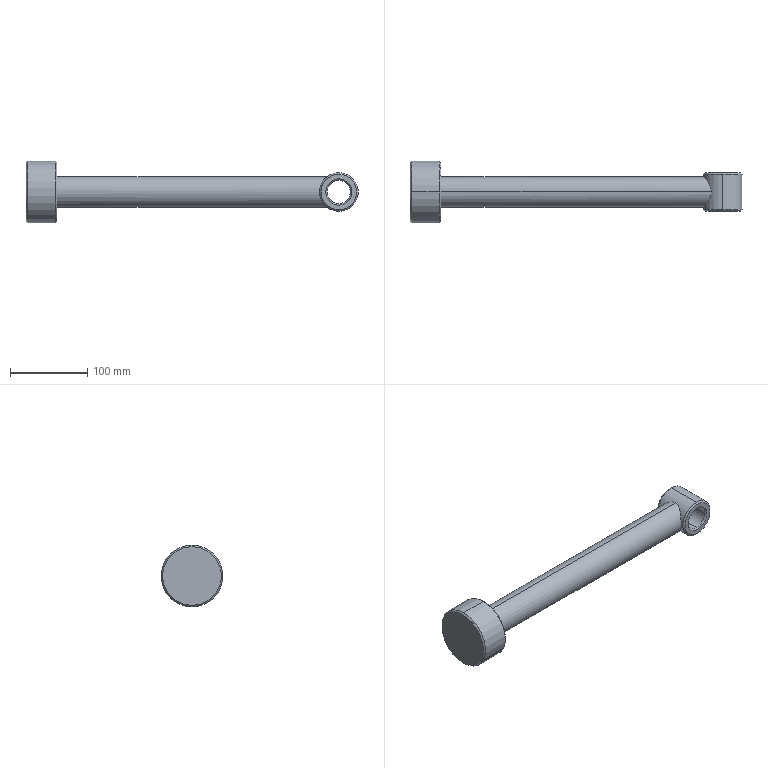Part | STEP file | Piston rod | 1 solid | 24 faces | box 430 x 80 x 80 mm | volume 691930 mm3 | cone 12 | cylinder 8 | plane 4 | commonest cylinder face diameters 30 x2 40 x2 50 x2 80 x2
STEP:
#1=CARTESIAN_POINT('',(405.,-23.,15.));
#2=VERTEX_POINT('',#1);
#3=CARTESIAN_POINT('',(405.,-23.,-15.));
#4=VERTEX_POINT('',#3);
#5=CARTESIAN_POINT('',(405.,-23.,0.));
#6=DIRECTION('',(0.,-1.,0.));
#7=DIRECTION('',(0.,0.,1.));
#8=AXIS2_PLACEMENT_3D('',#5,#6,#7);
#9=CIRCLE('',#8,15.);
#10=EDGE_CURVE('',#2,#4,#9,.T.);
#11=ORIENTED_EDGE('',*,*,#10,.F.);
#12=CARTESIAN_POINT('',(405.,-25.,17.));
#13=VERTEX_POINT('',#12);
#14=CARTESIAN_POINT('',(405.,-25.,17.));
#15=DIRECTION('',(0.,-0.7071,0.7071));
#16=VECTOR('',#15,1000.);
#17=LINE('',#14,#16);
#18=EDGE_CURVE('',#2,#13,#17,.T.);
#19=ORIENTED_EDGE('',*,*,#18,.T.);
#20=CARTESIAN_POINT('',(405.,-25.,-17.));
#21=VERTEX_POINT('',#20);
#22=CARTESIAN_POINT('',(405.,-25.,0.));
#23=DIRECTION('',(0.,1.,0.));
#24=DIRECTION('',(0.,0.,1.));
#25=AXIS2_PLACEMENT_3D('',#22,#23,#24);
#26=CIRCLE('',#25,17.);
#27=EDGE_CURVE('',#21,#13,#26,.T.);
#28=ORIENTED_EDGE('',*,*,#27,.F.);
#29=CARTESIAN_POINT('',(405.,-25.,-17.));
#30=DIRECTION('',(0.,-0.7071,-0.7071));
#31=VECTOR('',#30,1000.);
#32=LINE('',#29,#31);
#33=EDGE_CURVE('',#4,#21,#32,.T.);
#34=ORIENTED_EDGE('',*,*,#33,.F.);
#35=EDGE_LOOP('',(#11,#19,#28,#34));
#36=FACE_OUTER_BOUND('',#35,.T.);
#37=CARTESIAN_POINT('',(405.,-25.,0.));
#38=DIRECTION('',(0.,-1.,0.));
#39=DIRECTION('',(0.,0.,-1.));
#40=AXIS2_PLACEMENT_3D('',#37,#38,#39);
#41=CONICAL_SURFACE('',#40,17.,0.7854);
#42=ADVANCED_FACE('',(#36),#41,.F.);
#43=CARTESIAN_POINT('',(405.,-25.,-23.));
#44=VERTEX_POINT('',#43);
#45=CARTESIAN_POINT('',(405.,-25.,23.));
#46=VERTEX_POINT('',#45);
#47=CARTESIAN_POINT('',(405.,-25.,0.));
#48=DIRECTION('',(0.,-1.,0.));
#49=DIRECTION('',(0.,0.,1.));
#50=AXIS2_PLACEMENT_3D('',#47,#48,#49);
#51=CIRCLE('',#50,23.);
#52=EDGE_CURVE('',#44,#46,#51,.T.);
#53=ORIENTED_EDGE('',*,*,#52,.F.);
#54=CARTESIAN_POINT('',(405.,-23.,-25.));
#55=VERTEX_POINT('',#54);
#56=CARTESIAN_POINT('',(405.,-23.,-25.));
#57=DIRECTION('',(0.,0.7071,-0.7071));
#58=VECTOR('',#57,1000.);
#59=LINE('',#56,#58);
#60=EDGE_CURVE('',#44,#55,#59,.T.);
#61=ORIENTED_EDGE('',*,*,#60,.T.);
#62=CARTESIAN_POINT('',(405.,-23.,25.));
#63=VERTEX_POINT('',#62);
#64=CARTESIAN_POINT('',(405.,-23.,0.));
#65=DIRECTION('',(0.,1.,0.));
#66=DIRECTION('',(0.,0.,1.));
#67=AXIS2_PLACEMENT_3D('',#64,#65,#66);
#68=CIRCLE('',#67,25.);
#69=EDGE_CURVE('',#63,#55,#68,.T.);
#70=ORIENTED_EDGE('',*,*,#69,.F.);
#71=CARTESIAN_POINT('',(405.,-23.,25.));
#72=DIRECTION('',(0.,0.7071,0.7071));
#73=VECTOR('',#72,1000.);
#74=LINE('',#71,#73);
#75=EDGE_CURVE('',#46,#63,#74,.T.);
#76=ORIENTED_EDGE('',*,*,#75,.F.);
#77=EDGE_LOOP('',(#53,#61,#70,#76));
#78=FACE_OUTER_BOUND('',#77,.T.);
#79=CARTESIAN_POINT('',(405.,-23.,0.));
#80=DIRECTION('',(0.,1.,0.));
#81=DIRECTION('',(0.,0.,1.));
#82=AXIS2_PLACEMENT_3D('',#79,#80,#81);
#83=CONICAL_SURFACE('',#82,25.,0.7854);
#84=ADVANCED_FACE('',(#78),#83,.T.);
#85=CARTESIAN_POINT('',(405.,25.,23.));
#86=VERTEX_POINT('',#85);
#87=CARTESIAN_POINT('',(405.,25.,-23.));
#88=VERTEX_POINT('',#87);
#89=CARTESIAN_POINT('',(405.,25.,0.));
#90=DIRECTION('',(0.,1.,0.));
#91=DIRECTION('',(0.,0.,1.));
#92=AXIS2_PLACEMENT_3D('',#89,#90,#91);
#93=CIRCLE('',#92,23.);
#94=EDGE_CURVE('',#86,#88,#93,.T.);
#95=ORIENTED_EDGE('',*,*,#94,.F.);
#96=CARTESIAN_POINT('',(405.,23.,25.));
#97=VERTEX_POINT('',#96);
#98=CARTESIAN_POINT('',(405.,25.,23.));
#99=DIRECTION('',(0.,-0.7071,0.7071));
#100=VECTOR('',#99,1000.);
#101=LINE('',#98,#100);
#102=EDGE_CURVE('',#86,#97,#101,.T.);
#103=ORIENTED_EDGE('',*,*,#102,.T.);
#104=CARTESIAN_POINT('',(405.,23.,-25.));
#105=VERTEX_POINT('',#104);
#106=CARTESIAN_POINT('',(405.,23.,0.));
#107=DIRECTION('',(0.,-1.,0.));
#108=DIRECTION('',(0.,0.,1.));
#109=AXIS2_PLACEMENT_3D('',#106,#107,#108);
#110=CIRCLE('',#109,25.);
#111=EDGE_CURVE('',#105,#97,#110,.T.);
#112=ORIENTED_EDGE('',*,*,#111,.F.);
#113=CARTESIAN_POINT('',(405.,25.,-23.));
#114=DIRECTION('',(0.,-0.7071,-0.7071));
#115=VECTOR('',#114,1000.);
#116=LINE('',#113,#115);
#117=EDGE_CURVE('',#88,#105,#116,.T.);
#118=ORIENTED_EDGE('',*,*,#117,.F.);
#119=EDGE_LOOP('',(#95,#103,#112,#118));
#120=FACE_OUTER_BOUND('',#119,.T.);
#121=CARTESIAN_POINT('',(405.,25.,0.));
#122=DIRECTION('',(0.,-1.,0.));
#123=DIRECTION('',(0.,0.,-1.));
#124=AXIS2_PLACEMENT_3D('',#121,#122,#123);
#125=CONICAL_SURFACE('',#124,23.,0.7854);
#126=ADVANCED_FACE('',(#120),#125,.T.);
#127=CARTESIAN_POINT('',(405.,23.,-15.));
#128=VERTEX_POINT('',#127);
#129=CARTESIAN_POINT('',(405.,23.,15.));
#130=VERTEX_POINT('',#129);
#131=CARTESIAN_POINT('',(405.,23.,0.));
#132=DIRECTION('',(0.,1.,0.));
#133=DIRECTION('',(0.,0.,1.));
#134=AXIS2_PLACEMENT_3D('',#131,#132,#133);
#135=CIRCLE('',#134,15.);
#136=EDGE_CURVE('',#128,#130,#135,.T.);
#137=ORIENTED_EDGE('',*,*,#136,.F.);
#138=CARTESIAN_POINT('',(405.,25.,-17.));
#139=VERTEX_POINT('',#138);
#140=CARTESIAN_POINT('',(405.,23.,-15.));
#141=DIRECTION('',(0.,0.7071,-0.7071));
#142=VECTOR('',#141,1000.);
#143=LINE('',#140,#142);
#144=EDGE_CURVE('',#128,#139,#143,.T.);
#145=ORIENTED_EDGE('',*,*,#144,.T.);
#146=CARTESIAN_POINT('',(405.,25.,17.));
#147=VERTEX_POINT('',#146);
#148=CARTESIAN_POINT('',(405.,25.,0.));
#149=DIRECTION('',(0.,-1.,0.));
#150=DIRECTION('',(0.,0.,1.));
#151=AXIS2_PLACEMENT_3D('',#148,#149,#150);
#152=CIRCLE('',#151,17.);
#153=EDGE_CURVE('',#147,#139,#152,.T.);
#154=ORIENTED_EDGE('',*,*,#153,.F.);
#155=CARTESIAN_POINT('',(405.,23.,15.));
#156=DIRECTION('',(0.,0.7071,0.7071));
#157=VECTOR('',#156,1000.);
#158=LINE('',#155,#157);
#159=EDGE_CURVE('',#130,#147,#158,.T.);
#160=ORIENTED_EDGE('',*,*,#159,.F.);
#161=EDGE_LOOP('',(#137,#145,#154,#160));
#162=FACE_OUTER_BOUND('',#161,.T.);
#163=CARTESIAN_POINT('',(405.,23.,0.));
#164=DIRECTION('',(0.,1.,0.));
#165=DIRECTION('',(0.,0.,1.));
#166=AXIS2_PLACEMENT_3D('',#163,#164,#165);
#167=CONICAL_SURFACE('',#166,15.,0.7854);
#168=ADVANCED_FACE('',(#162),#167,.F.);
#169=CARTESIAN_POINT('',(40.,0.,-38.));
#170=VERTEX_POINT('',#169);
#171=CARTESIAN_POINT('',(40.,0.,38.));
#172=VERTEX_POINT('',#171);
#173=CARTESIAN_POINT('',(40.,0.,0.));
#174=DIRECTION('',(1.,0.,0.));
#175=DIRECTION('',(0.,0.,1.));
#176=AXIS2_PLACEMENT_3D('',#173,#174,#175);
#177=CIRCLE('',#176,38.);
#178=EDGE_CURVE('',#170,#172,#177,.T.);
#179=ORIENTED_EDGE('',*,*,#178,.F.);
#180=CARTESIAN_POINT('',(38.,0.,-40.));
#181=VERTEX_POINT('',#180);
#182=CARTESIAN_POINT('',(38.,0.,-40.));
#183=DIRECTION('',(-0.7071,0.,-0.7071));
#184=VECTOR('',#183,1000.);
#185=LINE('',#182,#184);
#186=EDGE_CURVE('',#170,#181,#185,.T.);
#187=ORIENTED_EDGE('',*,*,#186,.T.);
#188=CARTESIAN_POINT('',(38.,0.,40.));
#189=VERTEX_POINT('',#188);
#190=CARTESIAN_POINT('',(38.,0.,0.));
#191=DIRECTION('',(-1.,0.,0.));
#192=DIRECTION('',(0.,0.,1.));
#193=AXIS2_PLACEMENT_3D('',#190,#191,#192);
#194=CIRCLE('',#193,40.);
#195=EDGE_CURVE('',#189,#181,#194,.T.);
#196=ORIENTED_EDGE('',*,*,#195,.F.);
#197=CARTESIAN_POINT('',(38.,0.,40.));
#198=DIRECTION('',(-0.7071,0.,0.7071));
#199=VECTOR('',#198,1000.);
#200=LINE('',#197,#199);
#201=EDGE_CURVE('',#172,#189,#200,.T.);
#202=ORIENTED_EDGE('',*,*,#201,.F.);
#203=EDGE_LOOP('',(#179,#187,#196,#202));
#204=FACE_OUTER_BOUND('',#203,.T.);
#205=CARTESIAN_POINT('',(38.,0.,0.));
#206=DIRECTION('',(-1.,0.,0.));
#207=DIRECTION('',(0.,0.,1.));
#208=AXIS2_PLACEMENT_3D('',#205,#206,#207);
#209=CONICAL_SURFACE('',#208,40.,0.7854);
#210=ADVANCED_FACE('',(#204),#209,.T.);
#211=CARTESIAN_POINT('',(0.,0.,38.));
#212=VERTEX_POINT('',#211);
#213=CARTESIAN_POINT('',(0.,0.,-38.));
#214=VERTEX_POINT('',#213);
#215=CARTESIAN_POINT('',(0.,0.,0.));
#216=DIRECTION('',(-1.,0.,0.));
#217=DIRECTION('',(0.,0.,-1.));
#218=AXIS2_PLACEMENT_3D('',#215,#216,#217);
#219=CIRCLE('',#218,38.);
#220=EDGE_CURVE('',#212,#214,#219,.T.);
#221=ORIENTED_EDGE('',*,*,#220,.F.);
#222=CARTESIAN_POINT('',(2.,0.,40.));
#223=VERTEX_POINT('',#222);
#224=CARTESIAN_POINT('',(0.,0.,38.));
#225=DIRECTION('',(0.7071,0.,0.7071));
#226=VECTOR('',#225,1000.);
#227=LINE('',#224,#226);
#228=EDGE_CURVE('',#212,#223,#227,.T.);
#229=ORIENTED_EDGE('',*,*,#228,.T.);
#230=CARTESIAN_POINT('',(2.,0.,-40.));
#231=VERTEX_POINT('',#230);
#232=CARTESIAN_POINT('',(2.,0.,0.));
#233=DIRECTION('',(1.,0.,0.));
#234=DIRECTION('',(0.,0.,-1.));
#235=AXIS2_PLACEMENT_3D('',#232,#233,#234);
#236=CIRCLE('',#235,40.);
#237=EDGE_CURVE('',#231,#223,#236,.T.);
#238=ORIENTED_EDGE('',*,*,#237,.F.);
#239=CARTESIAN_POINT('',(0.,0.,-38.));
#240=DIRECTION('',(0.7071,0.,-0.7071));
#241=VECTOR('',#240,1000.);
#242=LINE('',#239,#241);
#243=EDGE_CURVE('',#214,#231,#242,.T.);
#244=ORIENTED_EDGE('',*,*,#243,.F.);
#245=EDGE_LOOP('',(#221,#229,#238,#244));
#246=FACE_OUTER_BOUND('',#245,.T.);
#247=CARTESIAN_POINT('',(0.,0.,0.));
#248=DIRECTION('',(1.,0.,0.));
#249=DIRECTION('',(0.,0.,-1.));
#250=AXIS2_PLACEMENT_3D('',#247,#248,#249);
#251=CONICAL_SURFACE('',#250,38.,0.7854);
#252=ADVANCED_FACE('',(#246),#251,.T.);
#253=ORIENTED_EDGE('',*,*,#10,.T.);
#254=CARTESIAN_POINT('',(405.,-25.,-15.));
#255=DIRECTION('',(0.,1.,0.));
#256=VECTOR('',#255,1000.);
#257=LINE('',#254,#256);
#258=EDGE_CURVE('',#4,#128,#257,.T.);
#259=ORIENTED_EDGE('',*,*,#258,.T.);
#260=ORIENTED_EDGE('',*,*,#136,.T.);
#261=CARTESIAN_POINT('',(405.,-25.,15.));
#262=DIRECTION('',(0.,1.,0.));
#263=VECTOR('',#262,1000.);
#264=LINE('',#261,#263);
#265=EDGE_CURVE('',#2,#130,#264,.T.);
#266=ORIENTED_EDGE('',*,*,#265,.F.);
#267=EDGE_LOOP('',(#253,#259,#260,#266));
#268=FACE_OUTER_BOUND('',#267,.T.);
#269=CARTESIAN_POINT('',(405.,-25.,0.));
#270=DIRECTION('',(0.,1.,0.));
#271=DIRECTION('',(0.,0.,1.));
#272=AXIS2_PLACEMENT_3D('',#269,#270,#271);
#273=CYLINDRICAL_SURFACE('',#272,15.);
#274=ADVANCED_FACE('',(#268),#273,.F.);
#275=ORIENTED_EDGE('',*,*,#69,.T.);
#276=CARTESIAN_POINT('',(405.,-25.,-25.));
#277=DIRECTION('',(0.,1.,0.));
#278=VECTOR('',#277,1000.);
#279=LINE('',#276,#278);
#280=EDGE_CURVE('',#55,#105,#279,.T.);
#281=ORIENTED_EDGE('',*,*,#280,.T.);
#282=ORIENTED_EDGE('',*,*,#111,.T.);
#283=CARTESIAN_POINT('',(405.,-25.,25.));
#284=DIRECTION('',(0.,1.,0.));
#285=VECTOR('',#284,1000.);
#286=LINE('',#283,#285);
#287=EDGE_CURVE('',#63,#97,#286,.T.);
#288=ORIENTED_EDGE('',*,*,#287,.F.);
#289=EDGE_LOOP('',(#275,#281,#282,#288));
#290=FACE_OUTER_BOUND('',#289,.T.);
#291=CARTESIAN_POINT('',(405.,-25.,0.));
#292=DIRECTION('',(0.,1.,0.));
#293=DIRECTION('',(0.,0.,1.));
#294=AXIS2_PLACEMENT_3D('',#291,#292,#293);
#295=CYLINDRICAL_SURFACE('',#294,25.);
#296=ADVANCED_FACE('',(#290),#295,.T.);
#297=CARTESIAN_POINT('',(390.,0.,20.));
#298=VERTEX_POINT('',#297);
#299=CARTESIAN_POINT('',(390.,0.,-20.));
#300=VERTEX_POINT('',#299);
#301=CARTESIAN_POINT('',(390.,0.,20.));
#302=CARTESIAN_POINT('',(390.,1.405,20.));
#303=CARTESIAN_POINT('',(389.801,2.765,19.854));
#304=CARTESIAN_POINT('',(389.366,4.419,19.509));
#305=CARTESIAN_POINT('',(389.27,4.748,19.431));
#306=CARTESIAN_POINT('',(389.064,5.391,19.263));
#307=CARTESIAN_POINT('',(388.954,5.707,19.171));
#308=CARTESIAN_POINT('',(388.606,6.639,18.877));
#309=CARTESIAN_POINT('',(388.352,7.241,18.654));
#310=CARTESIAN_POINT('',(387.81,8.412,18.156));
#311=CARTESIAN_POINT('',(387.524,8.98,17.882));
#312=CARTESIAN_POINT('',(386.929,10.089,17.281));
#313=CARTESIAN_POINT('',(386.624,10.624,16.957));
#314=CARTESIAN_POINT('',(385.704,12.167,15.922));
#315=CARTESIAN_POINT('',(385.083,13.119,15.147));
#316=CARTESIAN_POINT('',(384.176,14.448,13.844));
#317=CARTESIAN_POINT('',(383.878,14.873,13.386));
#318=CARTESIAN_POINT('',(383.295,15.69,12.418));
#319=CARTESIAN_POINT('',(383.013,16.078,11.913));
#320=CARTESIAN_POINT('',(382.208,17.167,10.341));
#321=CARTESIAN_POINT('',(381.725,17.8,9.215));
#322=CARTESIAN_POINT('',(381.21,18.465,7.692));
#323=CARTESIAN_POINT('',(381.112,18.592,7.38));
#324=CARTESIAN_POINT('',(380.927,18.829,6.751));
#325=CARTESIAN_POINT('',(380.84,18.94,6.433));
#326=CARTESIAN_POINT('',(380.597,19.249,5.471));
#327=CARTESIAN_POINT('',(380.459,19.423,4.817));
#328=CARTESIAN_POINT('',(380.235,19.706,3.483));
#329=CARTESIAN_POINT('',(380.148,19.815,2.803));
#330=CARTESIAN_POINT('',(380.03,19.962,1.415));
#331=CARTESIAN_POINT('',(380.001,19.999,0.7219));
#332=CARTESIAN_POINT('',(379.999,20.001,-0.6588));
#333=CARTESIAN_POINT('',(380.027,19.967,-1.347));
#334=CARTESIAN_POINT('',(380.111,19.861,-2.376));
#335=CARTESIAN_POINT('',(380.146,19.817,-2.719));
#336=CARTESIAN_POINT('',(380.23,19.711,-3.403));
#337=CARTESIAN_POINT('',(380.28,19.649,-3.745));
#338=CARTESIAN_POINT('',(380.558,19.298,-5.428));
#339=CARTESIAN_POINT('',(380.883,18.888,-6.71));
#340=CARTESIAN_POINT('',(381.394,18.227,-8.239));
#341=CARTESIAN_POINT('',(381.502,18.087,-8.541));
#342=CARTESIAN_POINT('',(381.726,17.796,-9.134));
#343=CARTESIAN_POINT('',(381.842,17.644,-9.424));
#344=CARTESIAN_POINT('',(382.202,17.17,-10.278));
#345=CARTESIAN_POINT('',(382.457,16.83,-10.824));
#346=CARTESIAN_POINT('',(382.993,16.105,-11.877));
#347=CARTESIAN_POINT('',(383.274,15.719,-12.382));
#348=CARTESIAN_POINT('',(383.858,14.903,-13.354));
#349=CARTESIAN_POINT('',(384.157,14.476,-13.815));
#350=CARTESIAN_POINT('',(385.066,13.144,-15.125));
#351=CARTESIAN_POINT('',(385.69,12.188,-15.906));
#352=CARTESIAN_POINT('',(386.616,10.636,-16.949));
#353=CARTESIAN_POINT('',(386.924,10.098,-17.275));
#354=CARTESIAN_POINT('',(387.516,8.995,-17.874));
#355=CARTESIAN_POINT('',(387.802,8.428,-18.149));
#356=CARTESIAN_POINT('',(388.344,7.258,-18.648));
#357=CARTESIAN_POINT('',(388.6,6.655,-18.872));
#358=CARTESIAN_POINT('',(389.066,5.406,-19.267));
#359=CARTESIAN_POINT('',(389.277,4.756,-19.438));
#360=CARTESIAN_POINT('',(389.624,3.439,-19.714));
#361=CARTESIAN_POINT('',(389.762,2.768,-19.819));
#362=CARTESIAN_POINT('',(389.903,1.742,-19.927));
#363=CARTESIAN_POINT('',(389.939,1.397,-19.954));
#364=CARTESIAN_POINT('',(389.988,0.698,-19.991));
#365=CARTESIAN_POINT('',(390.,0.3476,-20.));
#366=CARTESIAN_POINT('',(390.,0.,-20.));
#367=B_SPLINE_CURVE_WITH_KNOTS('',3,(#301,#302,#303,#304,#305,#306,#307,#308,#309,#310,#311,#312,#313,#314,#315,#316,#317,#318,#319,#320,#321,#322,#323,#324,#325,#326,#327,#328,#329,#330,#331,#332,#333,#334,#335,#336,#337,#338,#339,#340,#341,#342,#343,#344,#345,#346,#347,#348,#349,#350,#351,#352,#353,#354,#355,#356,#357,#358,#359,#360,#361,#362,#363,#364,#365,#366),.UNSPECIFIED.,.F.,.F.,(4,2,2,2,2,2,2,2,2,2,2,2,2,2,2,2,2,2,2,2,2,2,2,2,2,2,2,2,2,2,2,2,4),(0.,0.004146,0.005182,0.006219,0.008292,0.01036,0.01244,0.01658,0.01866,0.02073,0.02487,0.02591,0.02695,0.02902,0.03109,0.03317,0.03524,0.03628,0.03731,0.04146,0.04249,0.04353,0.0456,0.04768,0.04975,0.0539,0.05597,0.05804,0.06011,0.06219,0.06426,0.0653,0.06633),.UNSPECIFIED.);
#368=EDGE_CURVE('',#298,#300,#367,.T.);
#369=ORIENTED_EDGE('',*,*,#368,.T.);
#370=CARTESIAN_POINT('',(40.,0.,-20.));
#371=VERTEX_POINT('',#370);
#372=CARTESIAN_POINT('',(0.,0.,-20.));
#373=DIRECTION('',(-1.,0.,0.));
#374=VECTOR('',#373,1000.);
#375=LINE('',#372,#374);
#376=EDGE_CURVE('',#300,#371,#375,.T.);
#377=ORIENTED_EDGE('',*,*,#376,.T.);
#378=CARTESIAN_POINT('',(40.,0.,20.));
#379=VERTEX_POINT('',#378);
#380=CARTESIAN_POINT('',(40.,0.,0.));
#381=DIRECTION('',(-1.,0.,0.));
#382=DIRECTION('',(0.,0.,1.));
#383=AXIS2_PLACEMENT_3D('',#380,#381,#382);
#384=CIRCLE('',#383,20.);
#385=EDGE_CURVE('',#379,#371,#384,.T.);
#386=ORIENTED_EDGE('',*,*,#385,.F.);
#387=CARTESIAN_POINT('',(0.,0.,20.));
#388=DIRECTION('',(-1.,0.,0.));
#389=VECTOR('',#388,1000.);
#390=LINE('',#387,#389);
#391=EDGE_CURVE('',#298,#379,#390,.T.);
#392=ORIENTED_EDGE('',*,*,#391,.F.);
#393=EDGE_LOOP('',(#369,#377,#386,#392));
#394=FACE_OUTER_BOUND('',#393,.T.);
#395=CARTESIAN_POINT('',(0.,0.,0.));
#396=DIRECTION('',(-1.,0.,0.));
#397=DIRECTION('',(0.,0.,1.));
#398=AXIS2_PLACEMENT_3D('',#395,#396,#397);
#399=CYLINDRICAL_SURFACE('',#398,20.);
#400=ADVANCED_FACE('',(#394),#399,.T.);
#401=ORIENTED_EDGE('',*,*,#195,.T.);
#402=CARTESIAN_POINT('',(0.,0.,-40.));
#403=DIRECTION('',(-1.,0.,0.));
#404=VECTOR('',#403,1000.);
#405=LINE('',#402,#404);
#406=EDGE_CURVE('',#181,#231,#405,.T.);
#407=ORIENTED_EDGE('',*,*,#406,.T.);
#408=ORIENTED_EDGE('',*,*,#237,.T.);
#409=CARTESIAN_POINT('',(0.,0.,40.));
#410=DIRECTION('',(-1.,0.,0.));
#411=VECTOR('',#410,1000.);
#412=LINE('',#409,#411);
#413=EDGE_CURVE('',#189,#223,#412,.T.);
#414=ORIENTED_EDGE('',*,*,#413,.F.);
#415=EDGE_LOOP('',(#401,#407,#408,#414));
#416=FACE_OUTER_BOUND('',#415,.T.);
#417=CARTESIAN_POINT('',(0.,0.,0.));
#418=DIRECTION('',(-1.,0.,0.));
#419=DIRECTION('',(0.,0.,1.));
#420=AXIS2_PLACEMENT_3D('',#417,#418,#419);
#421=CYLINDRICAL_SURFACE('',#420,40.);
#422=ADVANCED_FACE('',(#416),#421,.T.);
#423=CARTESIAN_POINT('',(0.,0.,0.));
#424=DIRECTION('',(-1.,0.,0.));
#425=DIRECTION('',(0.,0.,-1.));
#426=AXIS2_PLACEMENT_3D('',#423,#424,#425);
#427=CIRCLE('',#426,38.);
#428=EDGE_CURVE('',#214,#212,#427,.T.);
#429=ORIENTED_EDGE('',*,*,#428,.T.);
#430=ORIENTED_EDGE('',*,*,#220,.T.);
#431=EDGE_LOOP('',(#429,#430));
#432=FACE_OUTER_BOUND('',#431,.T.);
#433=CARTESIAN_POINT('',(0.,0.,0.));
#434=DIRECTION('',(1.,0.,0.));
#435=DIRECTION('',(0.,0.,-1.));
#436=AXIS2_PLACEMENT_3D('',#433,#434,#435);
#437=PLANE('',#436);
#438=ADVANCED_FACE('',(#432),#437,.F.);
#439=ORIENTED_EDGE('',*,*,#406,.F.);
#440=CARTESIAN_POINT('',(38.,0.,0.));
#441=DIRECTION('',(-1.,0.,0.));
#442=DIRECTION('',(0.,0.,1.));
#443=AXIS2_PLACEMENT_3D('',#440,#441,#442);
#444=CIRCLE('',#443,40.);
#445=EDGE_CURVE('',#181,#189,#444,.T.);
#446=ORIENTED_EDGE('',*,*,#445,.T.);
#447=ORIENTED_EDGE('',*,*,#413,.T.);
#448=CARTESIAN_POINT('',(2.,0.,0.));
#449=DIRECTION('',(1.,0.,0.));
#450=DIRECTION('',(0.,0.,-1.));
#451=AXIS2_PLACEMENT_3D('',#448,#449,#450);
#452=CIRCLE('',#451,40.);
#453=EDGE_CURVE('',#223,#231,#452,.T.);
#454=ORIENTED_EDGE('',*,*,#453,.T.);
#455=EDGE_LOOP('',(#439,#446,#447,#454));
#456=FACE_OUTER_BOUND('',#455,.T.);
#457=CARTESIAN_POINT('',(0.,0.,0.));
#458=DIRECTION('',(-1.,0.,0.));
#459=DIRECTION('',(0.,0.,1.));
#460=AXIS2_PLACEMENT_3D('',#457,#458,#459);
#461=CYLINDRICAL_SURFACE('',#460,40.);
#462=ADVANCED_FACE('',(#456),#461,.T.);
#463=CARTESIAN_POINT('',(40.,0.,0.));
#464=DIRECTION('',(1.,0.,0.));
#465=DIRECTION('',(0.,0.,1.));
#466=AXIS2_PLACEMENT_3D('',#463,#464,#465);
#467=CIRCLE('',#466,38.);
#468=EDGE_CURVE('',#172,#170,#467,.T.);
#469=ORIENTED_EDGE('',*,*,#468,.T.);
#470=ORIENTED_EDGE('',*,*,#178,.T.);
#471=EDGE_LOOP('',(#469,#470));
#472=FACE_OUTER_BOUND('',#471,.T.);
#473=ORIENTED_EDGE('',*,*,#385,.T.);
#474=CARTESIAN_POINT('',(40.,0.,0.));
#475=DIRECTION('',(-1.,0.,0.));
#476=DIRECTION('',(0.,0.,1.));
#477=AXIS2_PLACEMENT_3D('',#474,#475,#476);
#478=CIRCLE('',#477,20.);
#479=EDGE_CURVE('',#371,#379,#478,.T.);
#480=ORIENTED_EDGE('',*,*,#479,.T.);
#481=EDGE_LOOP('',(#473,#480));
#482=FACE_BOUND('',#481,.T.);
#483=CARTESIAN_POINT('',(40.,40.,0.));
#484=DIRECTION('',(-1.,0.,0.));
#485=DIRECTION('',(0.,0.,1.));
#486=AXIS2_PLACEMENT_3D('',#483,#484,#485);
#487=PLANE('',#486);
#488=ADVANCED_FACE('',(#472,#482),#487,.F.);
#489=ORIENTED_EDGE('',*,*,#376,.F.);
#490=CARTESIAN_POINT('',(390.,0.,-20.));
#491=CARTESIAN_POINT('',(390.,-0.6946,-20.));
#492=CARTESIAN_POINT('',(389.952,-1.383,-19.964));
#493=CARTESIAN_POINT('',(389.812,-2.406,-19.858));
#494=CARTESIAN_POINT('',(389.754,-2.745,-19.814));
#495=CARTESIAN_POINT('',(389.618,-3.421,-19.708));
#496=CARTESIAN_POINT('',(389.54,-3.758,-19.647));
#497=CARTESIAN_POINT('',(389.106,-5.409,-19.302));
#498=CARTESIAN_POINT('',(388.628,-6.644,-18.908));
#499=CARTESIAN_POINT('',(387.812,-8.409,-18.158));
#500=CARTESIAN_POINT('',(387.522,-8.983,-17.88));
#501=CARTESIAN_POINT('',(386.931,-10.085,-17.283));
#502=CARTESIAN_POINT('',(386.628,-10.615,-16.962));
#503=CARTESIAN_POINT('',(385.712,-12.154,-15.932));
#504=CARTESIAN_POINT('',(385.09,-13.109,-15.156));
#505=CARTESIAN_POINT('',(384.177,-14.447,-13.845));
#506=CARTESIAN_POINT('',(383.876,-14.877,-13.382));
#507=CARTESIAN_POINT('',(383.298,-15.687,-12.423));
#508=CARTESIAN_POINT('',(383.019,-16.069,-11.924));
#509=CARTESIAN_POINT('',(382.22,-17.151,-10.366));
#510=CARTESIAN_POINT('',(381.737,-17.784,-9.247));
#511=CARTESIAN_POINT('',(381.221,-18.451,-7.725));
#512=CARTESIAN_POINT('',(381.122,-18.578,-7.414));
#513=CARTESIAN_POINT('',(380.936,-18.817,-6.785));
#514=CARTESIAN_POINT('',(380.849,-18.928,-6.468));
#515=CARTESIAN_POINT('',(380.605,-19.239,-5.505));
#516=CARTESIAN_POINT('',(380.466,-19.415,-4.851));
#517=CARTESIAN_POINT('',(380.239,-19.7,-3.517));
#518=CARTESIAN_POINT('',(380.152,-19.81,-2.835));
#519=CARTESIAN_POINT('',(380.032,-19.96,-1.447));
#520=CARTESIAN_POINT('',(380.002,-19.998,-0.7543));
#521=CARTESIAN_POINT('',(379.998,-20.002,0.6273));
#522=CARTESIAN_POINT('',(380.025,-19.969,1.316));
#523=CARTESIAN_POINT('',(380.108,-19.865,2.347));
#524=CARTESIAN_POINT('',(380.143,-19.821,2.69));
#525=CARTESIAN_POINT('',(380.227,-19.716,3.376));
#526=CARTESIAN_POINT('',(380.276,-19.654,3.718));
#527=CARTESIAN_POINT('',(380.553,-19.306,5.403));
#528=CARTESIAN_POINT('',(380.876,-18.897,6.686));
#529=CARTESIAN_POINT('',(381.387,-18.237,8.218));
#530=CARTESIAN_POINT('',(381.495,-18.097,8.521));
#531=CARTESIAN_POINT('',(381.718,-17.806,9.114));
#532=CARTESIAN_POINT('',(381.834,-17.654,9.405));
#533=CARTESIAN_POINT('',(382.194,-17.18,10.26));
#534=CARTESIAN_POINT('',(382.449,-16.841,10.807));
#535=CARTESIAN_POINT('',(382.985,-16.116,11.862));
#536=CARTESIAN_POINT('',(383.266,-15.73,12.368));
#537=CARTESIAN_POINT('',(383.85,-14.913,13.342));
#538=CARTESIAN_POINT('',(384.149,-14.487,13.803));
#539=CARTESIAN_POINT('',(385.059,-13.156,15.116));
#540=CARTESIAN_POINT('',(385.684,-12.199,15.898));
#541=CARTESIAN_POINT('',(386.611,-10.646,16.943));
#542=CARTESIAN_POINT('',(386.918,-10.107,17.269));
#543=CARTESIAN_POINT('',(387.511,-9.004,17.869));
#544=CARTESIAN_POINT('',(387.798,-8.437,18.144));
#545=CARTESIAN_POINT('',(388.341,-7.267,18.644));
#546=CARTESIAN_POINT('',(388.597,-6.664,18.869));
#547=CARTESIAN_POINT('',(389.064,-5.413,19.265));
#548=CARTESIAN_POINT('',(389.275,-4.763,19.436));
#549=CARTESIAN_POINT('',(389.622,-3.446,19.712));
#550=CARTESIAN_POINT('',(389.761,-2.775,19.818));
#551=CARTESIAN_POINT('',(389.902,-1.748,19.926));
#552=CARTESIAN_POINT('',(389.939,-1.403,19.954));
#553=CARTESIAN_POINT('',(389.988,-0.7036,19.991));
#554=CARTESIAN_POINT('',(390.,-0.3509,20.));
#555=CARTESIAN_POINT('',(390.,0.,20.));
#556=B_SPLINE_CURVE_WITH_KNOTS('',3,(#490,#491,#492,#493,#494,#495,#496,#497,#498,#499,#500,#501,#502,#503,#504,#505,#506,#507,#508,#509,#510,#511,#512,#513,#514,#515,#516,#517,#518,#519,#520,#521,#522,#523,#524,#525,#526,#527,#528,#529,#530,#531,#532,#533,#534,#535,#536,#537,#538,#539,#540,#541,#542,#543,#544,#545,#546,#547,#548,#549,#550,#551,#552,#553,#554,#555),.UNSPECIFIED.,.F.,.F.,(4,2,2,2,2,2,2,2,2,2,2,2,2,2,2,2,2,2,2,2,2,2,2,2,2,2,2,2,2,2,2,2,4),(0.06633,0.0684,0.06944,0.07048,0.07462,0.07669,0.07876,0.0829,0.08497,0.08705,0.09119,0.09222,0.09326,0.09533,0.0974,0.09947,0.1015,0.1026,0.1036,0.1078,0.1088,0.1098,0.1119,0.114,0.116,0.1202,0.1223,0.1243,0.1264,0.1285,0.1305,0.1316,0.1326),.UNSPECIFIED.);
#557=EDGE_CURVE('',#300,#298,#556,.T.);
#558=ORIENTED_EDGE('',*,*,#557,.T.);
#559=ORIENTED_EDGE('',*,*,#391,.T.);
#560=ORIENTED_EDGE('',*,*,#479,.F.);
#561=EDGE_LOOP('',(#489,#558,#559,#560));
#562=FACE_OUTER_BOUND('',#561,.T.);
#563=CARTESIAN_POINT('',(0.,0.,0.));
#564=DIRECTION('',(-1.,0.,0.));
#565=DIRECTION('',(0.,0.,1.));
#566=AXIS2_PLACEMENT_3D('',#563,#564,#565);
#567=CYLINDRICAL_SURFACE('',#566,20.);
#568=ADVANCED_FACE('',(#562),#567,.T.);
#569=ORIENTED_EDGE('',*,*,#280,.F.);
#570=CARTESIAN_POINT('',(405.,-23.,0.));
#571=DIRECTION('',(0.,1.,0.));
#572=DIRECTION('',(0.,0.,1.));
#573=AXIS2_PLACEMENT_3D('',#570,#571,#572);
#574=CIRCLE('',#573,25.);
#575=EDGE_CURVE('',#55,#63,#574,.T.);
#576=ORIENTED_EDGE('',*,*,#575,.T.);
#577=ORIENTED_EDGE('',*,*,#287,.T.);
#578=CARTESIAN_POINT('',(405.,23.,0.));
#579=DIRECTION('',(0.,-1.,0.));
#580=DIRECTION('',(0.,0.,1.));
#581=AXIS2_PLACEMENT_3D('',#578,#579,#580);
#582=CIRCLE('',#581,25.);
#583=EDGE_CURVE('',#97,#105,#582,.T.);
#584=ORIENTED_EDGE('',*,*,#583,.T.);
#585=EDGE_LOOP('',(#569,#576,#577,#584));
#586=FACE_OUTER_BOUND('',#585,.T.);
#587=ORIENTED_EDGE('',*,*,#368,.F.);
#588=ORIENTED_EDGE('',*,*,#557,.F.);
#589=EDGE_LOOP('',(#587,#588));
#590=FACE_BOUND('',#589,.T.);
#591=CARTESIAN_POINT('',(405.,-25.,0.));
#592=DIRECTION('',(0.,1.,0.));
#593=DIRECTION('',(0.,0.,1.));
#594=AXIS2_PLACEMENT_3D('',#591,#592,#593);
#595=CYLINDRICAL_SURFACE('',#594,25.);
#596=ADVANCED_FACE('',(#586,#590),#595,.T.);
#597=CARTESIAN_POINT('',(405.,-25.,0.));
#598=DIRECTION('',(0.,-1.,0.));
#599=DIRECTION('',(0.,0.,1.));
#600=AXIS2_PLACEMENT_3D('',#597,#598,#599);
#601=CIRCLE('',#600,23.);
#602=EDGE_CURVE('',#46,#44,#601,.T.);
#603=ORIENTED_EDGE('',*,*,#602,.T.);
#604=ORIENTED_EDGE('',*,*,#52,.T.);
#605=EDGE_LOOP('',(#603,#604));
#606=FACE_OUTER_BOUND('',#605,.T.);
#607=ORIENTED_EDGE('',*,*,#27,.T.);
#608=CARTESIAN_POINT('',(405.,-25.,0.));
#609=DIRECTION('',(0.,1.,0.));
#610=DIRECTION('',(0.,0.,1.));
#611=AXIS2_PLACEMENT_3D('',#608,#609,#610);
#612=CIRCLE('',#611,17.);
#613=EDGE_CURVE('',#13,#21,#612,.T.);
#614=ORIENTED_EDGE('',*,*,#613,.T.);
#615=EDGE_LOOP('',(#607,#614));
#616=FACE_BOUND('',#615,.T.);
#617=CARTESIAN_POINT('',(405.,-25.,0.));
#618=DIRECTION('',(0.,1.,0.));
#619=DIRECTION('',(0.,0.,1.));
#620=AXIS2_PLACEMENT_3D('',#617,#618,#619);
#621=PLANE('',#620);
#622=ADVANCED_FACE('',(#606,#616),#621,.F.);
#623=ORIENTED_EDGE('',*,*,#258,.F.);
#624=CARTESIAN_POINT('',(405.,-23.,0.));
#625=DIRECTION('',(0.,-1.,0.));
#626=DIRECTION('',(0.,0.,1.));
#627=AXIS2_PLACEMENT_3D('',#624,#625,#626);
#628=CIRCLE('',#627,15.);
#629=EDGE_CURVE('',#4,#2,#628,.T.);
#630=ORIENTED_EDGE('',*,*,#629,.T.);
#631=ORIENTED_EDGE('',*,*,#265,.T.);
#632=CARTESIAN_POINT('',(405.,23.,0.));
#633=DIRECTION('',(0.,1.,0.));
#634=DIRECTION('',(0.,0.,1.));
#635=AXIS2_PLACEMENT_3D('',#632,#633,#634);
#636=CIRCLE('',#635,15.);
#637=EDGE_CURVE('',#130,#128,#636,.T.);
#638=ORIENTED_EDGE('',*,*,#637,.T.);
#639=EDGE_LOOP('',(#623,#630,#631,#638));
#640=FACE_OUTER_BOUND('',#639,.T.);
#641=CARTESIAN_POINT('',(405.,-25.,0.));
#642=DIRECTION('',(0.,1.,0.));
#643=DIRECTION('',(0.,0.,1.));
#644=AXIS2_PLACEMENT_3D('',#641,#642,#643);
#645=CYLINDRICAL_SURFACE('',#644,15.);
#646=ADVANCED_FACE('',(#640),#645,.F.);
#647=ORIENTED_EDGE('',*,*,#153,.T.);
#648=CARTESIAN_POINT('',(405.,25.,0.));
#649=DIRECTION('',(0.,-1.,0.));
#650=DIRECTION('',(0.,0.,1.));
#651=AXIS2_PLACEMENT_3D('',#648,#649,#650);
#652=CIRCLE('',#651,17.);
#653=EDGE_CURVE('',#139,#147,#652,.T.);
#654=ORIENTED_EDGE('',*,*,#653,.T.);
#655=EDGE_LOOP('',(#647,#654));
#656=FACE_BOUND('',#655,.T.);
#657=CARTESIAN_POINT('',(405.,25.,0.));
#658=DIRECTION('',(0.,1.,0.));
#659=DIRECTION('',(0.,0.,1.));
#660=AXIS2_PLACEMENT_3D('',#657,#658,#659);
#661=CIRCLE('',#660,23.);
#662=EDGE_CURVE('',#88,#86,#661,.T.);
#663=ORIENTED_EDGE('',*,*,#662,.T.);
#664=ORIENTED_EDGE('',*,*,#94,.T.);
#665=EDGE_LOOP('',(#663,#664));
#666=FACE_OUTER_BOUND('',#665,.T.);
#667=CARTESIAN_POINT('',(405.,25.,0.));
#668=DIRECTION('',(0.,1.,0.));
#669=DIRECTION('',(0.,0.,1.));
#670=AXIS2_PLACEMENT_3D('',#667,#668,#669);
#671=PLANE('',#670);
#672=ADVANCED_FACE('',(#656,#666),#671,.T.);
#673=ORIENTED_EDGE('',*,*,#228,.F.);
#674=ORIENTED_EDGE('',*,*,#428,.F.);
#675=ORIENTED_EDGE('',*,*,#243,.T.);
#676=ORIENTED_EDGE('',*,*,#453,.F.);
#677=EDGE_LOOP('',(#673,#674,#675,#676));
#678=FACE_OUTER_BOUND('',#677,.T.);
#679=CARTESIAN_POINT('',(0.,0.,0.));
#680=DIRECTION('',(1.,0.,0.));
#681=DIRECTION('',(0.,0.,-1.));
#682=AXIS2_PLACEMENT_3D('',#679,#680,#681);
#683=CONICAL_SURFACE('',#682,38.,0.7854);
#684=ADVANCED_FACE('',(#678),#683,.T.);
#685=ORIENTED_EDGE('',*,*,#186,.F.);
#686=ORIENTED_EDGE('',*,*,#468,.F.);
#687=ORIENTED_EDGE('',*,*,#201,.T.);
#688=ORIENTED_EDGE('',*,*,#445,.F.);
#689=EDGE_LOOP('',(#685,#686,#687,#688));
#690=FACE_OUTER_BOUND('',#689,.T.);
#691=CARTESIAN_POINT('',(38.,0.,0.));
#692=DIRECTION('',(-1.,0.,0.));
#693=DIRECTION('',(0.,0.,1.));
#694=AXIS2_PLACEMENT_3D('',#691,#692,#693);
#695=CONICAL_SURFACE('',#694,40.,0.7854);
#696=ADVANCED_FACE('',(#690),#695,.T.);
#697=ORIENTED_EDGE('',*,*,#144,.F.);
#698=ORIENTED_EDGE('',*,*,#637,.F.);
#699=ORIENTED_EDGE('',*,*,#159,.T.);
#700=ORIENTED_EDGE('',*,*,#653,.F.);
#701=EDGE_LOOP('',(#697,#698,#699,#700));
#702=FACE_OUTER_BOUND('',#701,.T.);
#703=CARTESIAN_POINT('',(405.,23.,0.));
#704=DIRECTION('',(0.,1.,0.));
#705=DIRECTION('',(0.,0.,1.));
#706=AXIS2_PLACEMENT_3D('',#703,#704,#705);
#707=CONICAL_SURFACE('',#706,15.,0.7854);
#708=ADVANCED_FACE('',(#702),#707,.F.);
#709=ORIENTED_EDGE('',*,*,#102,.F.);
#710=ORIENTED_EDGE('',*,*,#662,.F.);
#711=ORIENTED_EDGE('',*,*,#117,.T.);
#712=ORIENTED_EDGE('',*,*,#583,.F.);
#713=EDGE_LOOP('',(#709,#710,#711,#712));
#714=FACE_OUTER_BOUND('',#713,.T.);
#715=CARTESIAN_POINT('',(405.,25.,0.));
#716=DIRECTION('',(0.,-1.,0.));
#717=DIRECTION('',(0.,0.,-1.));
#718=AXIS2_PLACEMENT_3D('',#715,#716,#717);
#719=CONICAL_SURFACE('',#718,23.,0.7854);
#720=ADVANCED_FACE('',(#714),#719,.T.);
#721=ORIENTED_EDGE('',*,*,#60,.F.);
#722=ORIENTED_EDGE('',*,*,#602,.F.);
#723=ORIENTED_EDGE('',*,*,#75,.T.);
#724=ORIENTED_EDGE('',*,*,#575,.F.);
#725=EDGE_LOOP('',(#721,#722,#723,#724));
#726=FACE_OUTER_BOUND('',#725,.T.);
#727=CARTESIAN_POINT('',(405.,-23.,0.));
#728=DIRECTION('',(0.,1.,0.));
#729=DIRECTION('',(0.,0.,1.));
#730=AXIS2_PLACEMENT_3D('',#727,#728,#729);
#731=CONICAL_SURFACE('',#730,25.,0.7854);
#732=ADVANCED_FACE('',(#726),#731,.T.);
#733=ORIENTED_EDGE('',*,*,#18,.F.);
#734=ORIENTED_EDGE('',*,*,#629,.F.);
#735=ORIENTED_EDGE('',*,*,#33,.T.);
#736=ORIENTED_EDGE('',*,*,#613,.F.);
#737=EDGE_LOOP('',(#733,#734,#735,#736));
#738=FACE_OUTER_BOUND('',#737,.T.);
#739=CARTESIAN_POINT('',(405.,-25.,0.));
#740=DIRECTION('',(0.,-1.,0.));
#741=DIRECTION('',(0.,0.,-1.));
#742=AXIS2_PLACEMENT_3D('',#739,#740,#741);
#743=CONICAL_SURFACE('',#742,17.,0.7854);
#744=ADVANCED_FACE('',(#738),#743,.F.);
#745=CLOSED_SHELL('',(#42,#84,#126,#168,#210,#252,#274,#296,#400,#422,#438,#462,#488,#568,#596,#622,#646,#672,#684,#696,#708,#720,#732,#744));
#746=MANIFOLD_SOLID_BREP('',#745);
#747=CARTESIAN_POINT('',(0.,0.,0.));
#748=DIRECTION('',(0.,0.,1.));
#749=DIRECTION('',(1.,0.,0.));
#750=AXIS2_PLACEMENT_3D('',#747,#748,#749);
#751=(LENGTH_UNIT()NAMED_UNIT(*)SI_UNIT(.MILLI.,.METRE.));
#752=UNCERTAINTY_MEASURE_WITH_UNIT(LENGTH_MEASURE(0.00001),#751,'','');
#753=(NAMED_UNIT(*)PLANE_ANGLE_UNIT()SI_UNIT($,.RADIAN.));
#754=(NAMED_UNIT(*)SI_UNIT($,.STERADIAN.)SOLID_ANGLE_UNIT());
#755=(GEOMETRIC_REPRESENTATION_CONTEXT(3)GLOBAL_UNCERTAINTY_ASSIGNED_CONTEXT((#752))GLOBAL_UNIT_ASSIGNED_CONTEXT((#751,#753,#754))REPRESENTATION_CONTEXT('',''));
#756=ADVANCED_BREP_SHAPE_REPRESENTATION('',(#746,#750),#755);